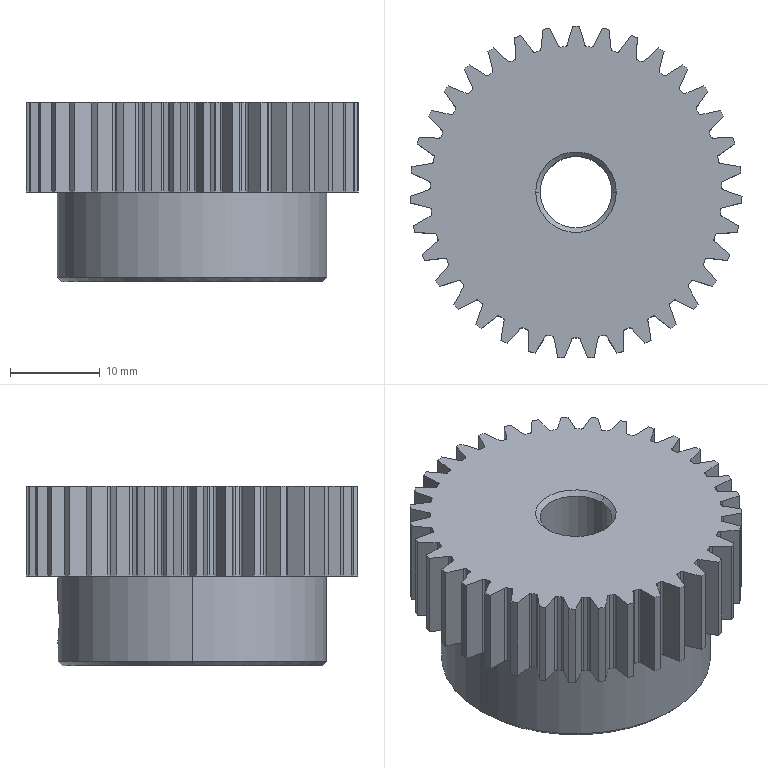Part | SolidWorks | features BaseBody 1 | 1 solid | 243 faces | box 36.989 x 36.955 x 20 mm | volume 15313 mm3 | cylinder 162 | plane 73 | cone 8 | commonest cylinder face diameters 0.5 x86 32.5 x35 37 x35 4.2 x2 8 x2 30 x2